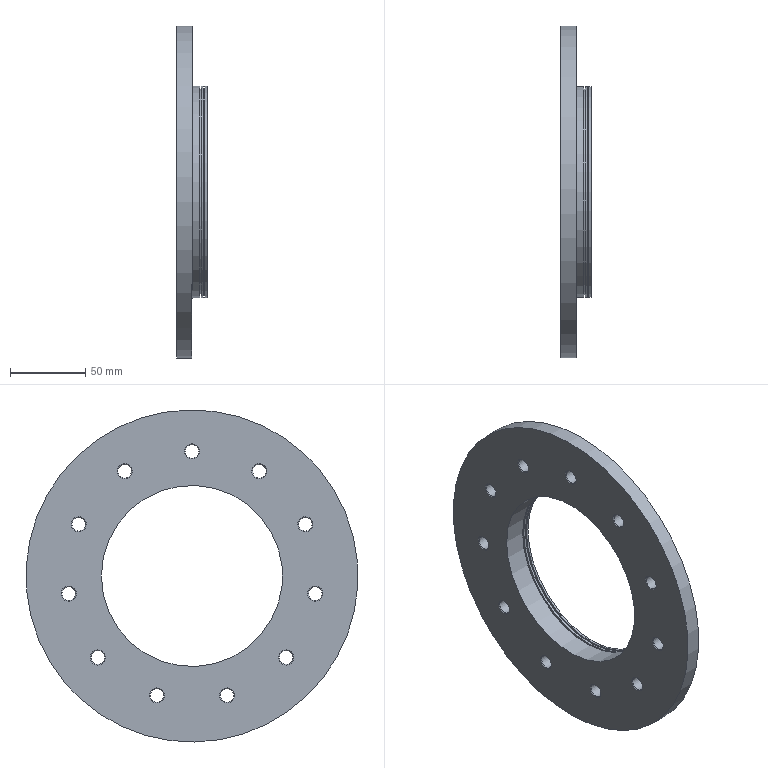Part | STEP file | Brake half | 1 solid | 46 faces | box 20 x 220 x 220 mm | volume 280546 mm3 | cylinder 23 | plane 12 | cone 11 | commonest cylinder face diameters 9 x11 120 x3 140 x3 124 x2 136 x2 177 x1
STEP:
#1=CARTESIAN_POINT('',(15.,0.,-70.));
#2=VERTEX_POINT('',#1);
#3=CARTESIAN_POINT('',(15.,0.,0.));
#4=DIRECTION('',(-1.,0.,0.));
#5=DIRECTION('',(0.,0.,-1.));
#6=AXIS2_PLACEMENT_3D('',#3,#4,#5);
#7=CIRCLE('',#6,70.);
#8=EDGE_CURVE('',#2,#2,#7,.T.);
#9=ORIENTED_EDGE('',*,*,#8,.T.);
#10=EDGE_LOOP('',(#9));
#11=FACE_OUTER_BOUND('',#10,.T.);
#12=CARTESIAN_POINT('',(8.,0.,-70.));
#13=VERTEX_POINT('',#12);
#14=CARTESIAN_POINT('',(8.,0.,0.));
#15=DIRECTION('',(1.,0.,0.));
#16=DIRECTION('',(0.,0.,-1.));
#17=AXIS2_PLACEMENT_3D('',#14,#15,#16);
#18=CIRCLE('',#17,70.);
#19=EDGE_CURVE('',#13,#13,#18,.T.);
#20=ORIENTED_EDGE('',*,*,#19,.T.);
#21=EDGE_LOOP('',(#20));
#22=FACE_OUTER_BOUND('',#21,.T.);
#23=CARTESIAN_POINT('',(20.,0.,0.));
#24=DIRECTION('',(-1.,0.,0.));
#25=DIRECTION('',(0.,0.,-1.));
#26=AXIS2_PLACEMENT_3D('',#23,#24,#25);
#27=CYLINDRICAL_SURFACE('',#26,70.);
#28=ADVANCED_FACE('',(#11,#22),#27,.T.);
#29=CARTESIAN_POINT('',(8.,-73.175,38.365));
#30=VERTEX_POINT('',#29);
#31=CARTESIAN_POINT('',(8.,-75.045,34.272));
#32=DIRECTION('',(1.,0.,0.));
#33=DIRECTION('',(0.,0.4154,0.9096));
#34=AXIS2_PLACEMENT_3D('',#31,#32,#33);
#35=CIRCLE('',#34,4.5);
#36=EDGE_CURVE('',#30,#30,#35,.T.);
#37=ORIENTED_EDGE('',*,*,#36,.T.);
#38=EDGE_LOOP('',(#37));
#39=FACE_OUTER_BOUND('',#38,.T.);
#40=CARTESIAN_POINT('',(0.5,-73.175,38.365));
#41=VERTEX_POINT('',#40);
#42=CARTESIAN_POINT('',(0.5,-75.045,34.272));
#43=DIRECTION('',(1.,0.,0.));
#44=DIRECTION('',(0.,0.4154,0.9096));
#45=AXIS2_PLACEMENT_3D('',#42,#43,#44);
#46=CIRCLE('',#45,4.5);
#47=EDGE_CURVE('',#41,#41,#46,.T.);
#48=ORIENTED_EDGE('',*,*,#47,.F.);
#49=EDGE_LOOP('',(#48));
#50=FACE_OUTER_BOUND('',#49,.T.);
#51=CARTESIAN_POINT('',(-30.,-75.045,34.272));
#52=DIRECTION('',(1.,0.,0.));
#53=DIRECTION('',(0.,0.4154,0.9096));
#54=AXIS2_PLACEMENT_3D('',#51,#52,#53);
#55=CYLINDRICAL_SURFACE('',#54,4.5);
#56=ADVANCED_FACE('',(#39,#50),#55,.F.);
#57=CARTESIAN_POINT('',(8.,-65.296,-50.625));
#58=VERTEX_POINT('',#57);
#59=CARTESIAN_POINT('',(8.,-62.349,-54.026));
#60=DIRECTION('',(1.,0.,0.));
#61=DIRECTION('',(0.,-0.6549,0.7557));
#62=AXIS2_PLACEMENT_3D('',#59,#60,#61);
#63=CIRCLE('',#62,4.5);
#64=EDGE_CURVE('',#58,#58,#63,.T.);
#65=ORIENTED_EDGE('',*,*,#64,.T.);
#66=EDGE_LOOP('',(#65));
#67=FACE_OUTER_BOUND('',#66,.T.);
#68=CARTESIAN_POINT('',(0.5,-65.296,-50.625));
#69=VERTEX_POINT('',#68);
#70=CARTESIAN_POINT('',(0.5,-62.349,-54.026));
#71=DIRECTION('',(1.,0.,0.));
#72=DIRECTION('',(0.,-0.6549,0.7557));
#73=AXIS2_PLACEMENT_3D('',#70,#71,#72);
#74=CIRCLE('',#73,4.5);
#75=EDGE_CURVE('',#69,#69,#74,.T.);
#76=ORIENTED_EDGE('',*,*,#75,.F.);
#77=EDGE_LOOP('',(#76));
#78=FACE_OUTER_BOUND('',#77,.T.);
#79=CARTESIAN_POINT('',(-30.,-62.349,-54.026));
#80=DIRECTION('',(1.,0.,0.));
#81=DIRECTION('',(0.,-0.6549,0.7557));
#82=AXIS2_PLACEMENT_3D('',#79,#80,#81);
#83=CYLINDRICAL_SURFACE('',#82,4.5);
#84=ADVANCED_FACE('',(#67,#78),#83,.F.);
#85=CARTESIAN_POINT('',(8.,18.925,-80.426));
#86=VERTEX_POINT('',#85);
#87=CARTESIAN_POINT('',(8.,23.243,-79.158));
#88=DIRECTION('',(1.,0.,0.));
#89=DIRECTION('',(0.,-0.9595,-0.2817));
#90=AXIS2_PLACEMENT_3D('',#87,#88,#89);
#91=CIRCLE('',#90,4.5);
#92=EDGE_CURVE('',#86,#86,#91,.T.);
#93=ORIENTED_EDGE('',*,*,#92,.T.);
#94=EDGE_LOOP('',(#93));
#95=FACE_OUTER_BOUND('',#94,.T.);
#96=CARTESIAN_POINT('',(0.5,18.925,-80.426));
#97=VERTEX_POINT('',#96);
#98=CARTESIAN_POINT('',(0.5,23.243,-79.158));
#99=DIRECTION('',(1.,0.,0.));
#100=DIRECTION('',(0.,-0.9595,-0.2817));
#101=AXIS2_PLACEMENT_3D('',#98,#99,#100);
#102=CIRCLE('',#101,4.5);
#103=EDGE_CURVE('',#97,#97,#102,.T.);
#104=ORIENTED_EDGE('',*,*,#103,.F.);
#105=EDGE_LOOP('',(#104));
#106=FACE_OUTER_BOUND('',#105,.T.);
#107=CARTESIAN_POINT('',(-30.,23.243,-79.158));
#108=DIRECTION('',(1.,0.,0.));
#109=DIRECTION('',(0.,-0.9595,-0.2817));
#110=AXIS2_PLACEMENT_3D('',#107,#108,#109);
#111=CYLINDRICAL_SURFACE('',#110,4.5);
#112=ADVANCED_FACE('',(#95,#106),#111,.F.);
#113=CARTESIAN_POINT('',(8.,81.02,-16.195));
#114=VERTEX_POINT('',#113);
#115=CARTESIAN_POINT('',(8.,81.66,-11.741));
#116=DIRECTION('',(1.,0.,0.));
#117=DIRECTION('',(0.,-0.1423,-0.9898));
#118=AXIS2_PLACEMENT_3D('',#115,#116,#117);
#119=CIRCLE('',#118,4.5);
#120=EDGE_CURVE('',#114,#114,#119,.T.);
#121=ORIENTED_EDGE('',*,*,#120,.T.);
#122=EDGE_LOOP('',(#121));
#123=FACE_OUTER_BOUND('',#122,.T.);
#124=CARTESIAN_POINT('',(0.5,81.02,-16.195));
#125=VERTEX_POINT('',#124);
#126=CARTESIAN_POINT('',(0.5,81.66,-11.741));
#127=DIRECTION('',(1.,0.,0.));
#128=DIRECTION('',(0.,-0.1423,-0.9898));
#129=AXIS2_PLACEMENT_3D('',#126,#127,#128);
#130=CIRCLE('',#129,4.5);
#131=EDGE_CURVE('',#125,#125,#130,.T.);
#132=ORIENTED_EDGE('',*,*,#131,.F.);
#133=EDGE_LOOP('',(#132));
#134=FACE_OUTER_BOUND('',#133,.T.);
#135=CARTESIAN_POINT('',(-30.,81.66,-11.741));
#136=DIRECTION('',(1.,0.,0.));
#137=DIRECTION('',(0.,-0.1423,-0.9898));
#138=AXIS2_PLACEMENT_3D('',#135,#136,#137);
#139=CYLINDRICAL_SURFACE('',#138,4.5);
#140=ADVANCED_FACE('',(#123,#134),#139,.F.);
#141=CARTESIAN_POINT('',(8.,48.389,66.971));
#142=VERTEX_POINT('',#141);
#143=CARTESIAN_POINT('',(8.,44.603,69.403));
#144=DIRECTION('',(1.,0.,0.));
#145=DIRECTION('',(0.,0.8413,-0.5406));
#146=AXIS2_PLACEMENT_3D('',#143,#144,#145);
#147=CIRCLE('',#146,4.5);
#148=EDGE_CURVE('',#142,#142,#147,.T.);
#149=ORIENTED_EDGE('',*,*,#148,.T.);
#150=EDGE_LOOP('',(#149));
#151=FACE_OUTER_BOUND('',#150,.T.);
#152=CARTESIAN_POINT('',(0.5,48.389,66.971));
#153=VERTEX_POINT('',#152);
#154=CARTESIAN_POINT('',(0.5,44.603,69.403));
#155=DIRECTION('',(1.,0.,0.));
#156=DIRECTION('',(0.,0.8413,-0.5406));
#157=AXIS2_PLACEMENT_3D('',#154,#155,#156);
#158=CIRCLE('',#157,4.5);
#159=EDGE_CURVE('',#153,#153,#158,.T.);
#160=ORIENTED_EDGE('',*,*,#159,.F.);
#161=EDGE_LOOP('',(#160));
#162=FACE_OUTER_BOUND('',#161,.T.);
#163=CARTESIAN_POINT('',(-30.,44.603,69.403));
#164=DIRECTION('',(1.,0.,0.));
#165=DIRECTION('',(0.,0.8413,-0.5406));
#166=AXIS2_PLACEMENT_3D('',#163,#164,#165);
#167=CYLINDRICAL_SURFACE('',#166,4.5);
#168=ADVANCED_FACE('',(#151,#162),#167,.F.);
#169=CARTESIAN_POINT('',(8.,76.914,30.178));
#170=VERTEX_POINT('',#169);
#171=CARTESIAN_POINT('',(8.,75.045,34.272));
#172=DIRECTION('',(1.,0.,0.));
#173=DIRECTION('',(0.,0.4154,-0.9096));
#174=AXIS2_PLACEMENT_3D('',#171,#172,#173);
#175=CIRCLE('',#174,4.5);
#176=EDGE_CURVE('',#170,#170,#175,.T.);
#177=ORIENTED_EDGE('',*,*,#176,.T.);
#178=EDGE_LOOP('',(#177));
#179=FACE_OUTER_BOUND('',#178,.T.);
#180=CARTESIAN_POINT('',(0.5,76.914,30.178));
#181=VERTEX_POINT('',#180);
#182=CARTESIAN_POINT('',(0.5,75.045,34.272));
#183=DIRECTION('',(1.,0.,0.));
#184=DIRECTION('',(0.,0.4154,-0.9096));
#185=AXIS2_PLACEMENT_3D('',#182,#183,#184);
#186=CIRCLE('',#185,4.5);
#187=EDGE_CURVE('',#181,#181,#186,.T.);
#188=ORIENTED_EDGE('',*,*,#187,.F.);
#189=EDGE_LOOP('',(#188));
#190=FACE_OUTER_BOUND('',#189,.T.);
#191=CARTESIAN_POINT('',(-30.,75.045,34.272));
#192=DIRECTION('',(1.,0.,0.));
#193=DIRECTION('',(0.,0.4154,-0.9096));
#194=AXIS2_PLACEMENT_3D('',#191,#192,#193);
#195=CYLINDRICAL_SURFACE('',#194,4.5);
#196=ADVANCED_FACE('',(#179,#190),#195,.F.);
#197=CARTESIAN_POINT('',(8.,59.402,-57.427));
#198=VERTEX_POINT('',#197);
#199=CARTESIAN_POINT('',(8.,62.349,-54.026));
#200=DIRECTION('',(1.,0.,0.));
#201=DIRECTION('',(0.,-0.6549,-0.7557));
#202=AXIS2_PLACEMENT_3D('',#199,#200,#201);
#203=CIRCLE('',#202,4.5);
#204=EDGE_CURVE('',#198,#198,#203,.T.);
#205=ORIENTED_EDGE('',*,*,#204,.T.);
#206=EDGE_LOOP('',(#205));
#207=FACE_OUTER_BOUND('',#206,.T.);
#208=CARTESIAN_POINT('',(0.5,59.402,-57.427));
#209=VERTEX_POINT('',#208);
#210=CARTESIAN_POINT('',(0.5,62.349,-54.026));
#211=DIRECTION('',(1.,0.,0.));
#212=DIRECTION('',(0.,-0.6549,-0.7557));
#213=AXIS2_PLACEMENT_3D('',#210,#211,#212);
#214=CIRCLE('',#213,4.5);
#215=EDGE_CURVE('',#209,#209,#214,.T.);
#216=ORIENTED_EDGE('',*,*,#215,.F.);
#217=EDGE_LOOP('',(#216));
#218=FACE_OUTER_BOUND('',#217,.T.);
#219=CARTESIAN_POINT('',(-30.,62.349,-54.026));
#220=DIRECTION('',(1.,0.,0.));
#221=DIRECTION('',(0.,-0.6549,-0.7557));
#222=AXIS2_PLACEMENT_3D('',#219,#220,#221);
#223=CYLINDRICAL_SURFACE('',#222,4.5);
#224=ADVANCED_FACE('',(#207,#218),#223,.F.);
#225=CARTESIAN_POINT('',(8.,-27.561,-77.89));
#226=VERTEX_POINT('',#225);
#227=CARTESIAN_POINT('',(8.,-23.243,-79.158));
#228=DIRECTION('',(1.,0.,0.));
#229=DIRECTION('',(0.,-0.9595,0.2817));
#230=AXIS2_PLACEMENT_3D('',#227,#228,#229);
#231=CIRCLE('',#230,4.5);
#232=EDGE_CURVE('',#226,#226,#231,.T.);
#233=ORIENTED_EDGE('',*,*,#232,.T.);
#234=EDGE_LOOP('',(#233));
#235=FACE_OUTER_BOUND('',#234,.T.);
#236=CARTESIAN_POINT('',(0.5,-27.561,-77.89));
#237=VERTEX_POINT('',#236);
#238=CARTESIAN_POINT('',(0.5,-23.243,-79.158));
#239=DIRECTION('',(1.,0.,0.));
#240=DIRECTION('',(0.,-0.9595,0.2817));
#241=AXIS2_PLACEMENT_3D('',#238,#239,#240);
#242=CIRCLE('',#241,4.5);
#243=EDGE_CURVE('',#237,#237,#242,.T.);
#244=ORIENTED_EDGE('',*,*,#243,.F.);
#245=EDGE_LOOP('',(#244));
#246=FACE_OUTER_BOUND('',#245,.T.);
#247=CARTESIAN_POINT('',(-30.,-23.243,-79.158));
#248=DIRECTION('',(1.,0.,0.));
#249=DIRECTION('',(0.,-0.9595,0.2817));
#250=AXIS2_PLACEMENT_3D('',#247,#248,#249);
#251=CYLINDRICAL_SURFACE('',#250,4.5);
#252=ADVANCED_FACE('',(#235,#246),#251,.F.);
#253=CARTESIAN_POINT('',(8.,-82.301,-7.287));
#254=VERTEX_POINT('',#253);
#255=CARTESIAN_POINT('',(8.,-81.66,-11.741));
#256=DIRECTION('',(1.,0.,0.));
#257=DIRECTION('',(0.,-0.1423,0.9898));
#258=AXIS2_PLACEMENT_3D('',#255,#256,#257);
#259=CIRCLE('',#258,4.5);
#260=EDGE_CURVE('',#254,#254,#259,.T.);
#261=ORIENTED_EDGE('',*,*,#260,.T.);
#262=EDGE_LOOP('',(#261));
#263=FACE_OUTER_BOUND('',#262,.T.);
#264=CARTESIAN_POINT('',(0.5,-82.301,-7.287));
#265=VERTEX_POINT('',#264);
#266=CARTESIAN_POINT('',(0.5,-81.66,-11.741));
#267=DIRECTION('',(1.,0.,0.));
#268=DIRECTION('',(0.,-0.1423,0.9898));
#269=AXIS2_PLACEMENT_3D('',#266,#267,#268);
#270=CIRCLE('',#269,4.5);
#271=EDGE_CURVE('',#265,#265,#270,.T.);
#272=ORIENTED_EDGE('',*,*,#271,.F.);
#273=EDGE_LOOP('',(#272));
#274=FACE_OUTER_BOUND('',#273,.T.);
#275=CARTESIAN_POINT('',(-30.,-81.66,-11.741));
#276=DIRECTION('',(1.,0.,0.));
#277=DIRECTION('',(0.,-0.1423,0.9898));
#278=AXIS2_PLACEMENT_3D('',#275,#276,#277);
#279=CYLINDRICAL_SURFACE('',#278,4.5);
#280=ADVANCED_FACE('',(#263,#274),#279,.F.);
#281=CARTESIAN_POINT('',(8.,-40.817,71.836));
#282=VERTEX_POINT('',#281);
#283=CARTESIAN_POINT('',(8.,-44.603,69.403));
#284=DIRECTION('',(1.,0.,0.));
#285=DIRECTION('',(0.,0.8413,0.5406));
#286=AXIS2_PLACEMENT_3D('',#283,#284,#285);
#287=CIRCLE('',#286,4.5);
#288=EDGE_CURVE('',#282,#282,#287,.T.);
#289=ORIENTED_EDGE('',*,*,#288,.T.);
#290=EDGE_LOOP('',(#289));
#291=FACE_OUTER_BOUND('',#290,.T.);
#292=CARTESIAN_POINT('',(0.5,-40.817,71.836));
#293=VERTEX_POINT('',#292);
#294=CARTESIAN_POINT('',(0.5,-44.603,69.403));
#295=DIRECTION('',(1.,0.,0.));
#296=DIRECTION('',(0.,0.8413,0.5406));
#297=AXIS2_PLACEMENT_3D('',#294,#295,#296);
#298=CIRCLE('',#297,4.5);
#299=EDGE_CURVE('',#293,#293,#298,.T.);
#300=ORIENTED_EDGE('',*,*,#299,.F.);
#301=EDGE_LOOP('',(#300));
#302=FACE_OUTER_BOUND('',#301,.T.);
#303=CARTESIAN_POINT('',(-30.,-44.603,69.403));
#304=DIRECTION('',(1.,0.,0.));
#305=DIRECTION('',(0.,0.8413,0.5406));
#306=AXIS2_PLACEMENT_3D('',#303,#304,#305);
#307=CYLINDRICAL_SURFACE('',#306,4.5);
#308=ADVANCED_FACE('',(#291,#302),#307,.F.);
#309=CARTESIAN_POINT('',(8.,4.5,82.5));
#310=VERTEX_POINT('',#309);
#311=CARTESIAN_POINT('',(8.,0.,82.5));
#312=DIRECTION('',(1.,0.,0.));
#313=DIRECTION('',(0.,1.,0.));
#314=AXIS2_PLACEMENT_3D('',#311,#312,#313);
#315=CIRCLE('',#314,4.5);
#316=EDGE_CURVE('',#310,#310,#315,.T.);
#317=ORIENTED_EDGE('',*,*,#316,.T.);
#318=EDGE_LOOP('',(#317));
#319=FACE_OUTER_BOUND('',#318,.T.);
#320=CARTESIAN_POINT('',(0.5,4.5,82.5));
#321=VERTEX_POINT('',#320);
#322=CARTESIAN_POINT('',(0.5,0.,82.5));
#323=DIRECTION('',(1.,0.,0.));
#324=DIRECTION('',(0.,1.,0.));
#325=AXIS2_PLACEMENT_3D('',#322,#323,#324);
#326=CIRCLE('',#325,4.5);
#327=EDGE_CURVE('',#321,#321,#326,.T.);
#328=ORIENTED_EDGE('',*,*,#327,.F.);
#329=EDGE_LOOP('',(#328));
#330=FACE_OUTER_BOUND('',#329,.T.);
#331=CARTESIAN_POINT('',(-30.,0.,82.5));
#332=DIRECTION('',(1.,0.,0.));
#333=DIRECTION('',(0.,1.,0.));
#334=AXIS2_PLACEMENT_3D('',#331,#332,#333);
#335=CYLINDRICAL_SURFACE('',#334,4.5);
#336=ADVANCED_FACE('',(#319,#330),#335,.F.);
#337=CARTESIAN_POINT('',(10.,-109.545,10.));
#338=VERTEX_POINT('',#337);
#339=CARTESIAN_POINT('',(10.,0.,0.));
#340=DIRECTION('',(1.,0.,0.));
#341=DIRECTION('',(0.,0.,-1.));
#342=AXIS2_PLACEMENT_3D('',#339,#340,#341);
#343=CIRCLE('',#342,110.);
#344=EDGE_CURVE('',#338,#338,#343,.T.);
#345=ORIENTED_EDGE('',*,*,#344,.T.);
#346=EDGE_LOOP('',(#345));
#347=FACE_BOUND('',#346,.T.);
#348=CARTESIAN_POINT('',(10.,0.,-88.5));
#349=VERTEX_POINT('',#348);
#350=CARTESIAN_POINT('',(10.,0.,0.));
#351=DIRECTION('',(1.,0.,0.));
#352=DIRECTION('',(0.,0.,-1.));
#353=AXIS2_PLACEMENT_3D('',#350,#351,#352);
#354=CIRCLE('',#353,88.5);
#355=EDGE_CURVE('',#349,#349,#354,.F.);
#356=ORIENTED_EDGE('',*,*,#355,.T.);
#357=EDGE_LOOP('',(#356));
#358=FACE_BOUND('',#357,.T.);
#359=CARTESIAN_POINT('',(10.,0.,0.));
#360=DIRECTION('',(1.,0.,0.));
#361=DIRECTION('',(0.,0.,-1.));
#362=AXIS2_PLACEMENT_3D('',#359,#360,#361);
#363=PLANE('',#362);
#364=ADVANCED_FACE('',(#347,#358),#363,.T.);
#365=ORIENTED_EDGE('',*,*,#355,.F.);
#366=EDGE_LOOP('',(#365));
#367=FACE_OUTER_BOUND('',#366,.T.);
#368=CARTESIAN_POINT('',(8.,0.,-88.5));
#369=VERTEX_POINT('',#368);
#370=CARTESIAN_POINT('',(8.,0.,0.));
#371=DIRECTION('',(1.,0.,0.));
#372=DIRECTION('',(0.,0.,-1.));
#373=AXIS2_PLACEMENT_3D('',#370,#371,#372);
#374=CIRCLE('',#373,88.5);
#375=EDGE_CURVE('',#369,#369,#374,.T.);
#376=ORIENTED_EDGE('',*,*,#375,.F.);
#377=EDGE_LOOP('',(#376));
#378=FACE_OUTER_BOUND('',#377,.T.);
#379=CARTESIAN_POINT('',(8.,0.,0.));
#380=DIRECTION('',(1.,0.,0.));
#381=DIRECTION('',(0.,0.,-1.));
#382=AXIS2_PLACEMENT_3D('',#379,#380,#381);
#383=CYLINDRICAL_SURFACE('',#382,88.5);
#384=ADVANCED_FACE('',(#367,#378),#383,.F.);
#385=ORIENTED_EDGE('',*,*,#375,.T.);
#386=EDGE_LOOP('',(#385));
#387=FACE_BOUND('',#386,.T.);
#388=ORIENTED_EDGE('',*,*,#316,.F.);
#389=EDGE_LOOP('',(#388));
#390=FACE_BOUND('',#389,.T.);
#391=ORIENTED_EDGE('',*,*,#288,.F.);
#392=EDGE_LOOP('',(#391));
#393=FACE_BOUND('',#392,.T.);
#394=ORIENTED_EDGE('',*,*,#260,.F.);
#395=EDGE_LOOP('',(#394));
#396=FACE_BOUND('',#395,.T.);
#397=ORIENTED_EDGE('',*,*,#232,.F.);
#398=EDGE_LOOP('',(#397));
#399=FACE_BOUND('',#398,.T.);
#400=ORIENTED_EDGE('',*,*,#204,.F.);
#401=EDGE_LOOP('',(#400));
#402=FACE_BOUND('',#401,.T.);
#403=ORIENTED_EDGE('',*,*,#176,.F.);
#404=EDGE_LOOP('',(#403));
#405=FACE_BOUND('',#404,.T.);
#406=ORIENTED_EDGE('',*,*,#148,.F.);
#407=EDGE_LOOP('',(#406));
#408=FACE_BOUND('',#407,.T.);
#409=ORIENTED_EDGE('',*,*,#120,.F.);
#410=EDGE_LOOP('',(#409));
#411=FACE_BOUND('',#410,.T.);
#412=ORIENTED_EDGE('',*,*,#92,.F.);
#413=EDGE_LOOP('',(#412));
#414=FACE_BOUND('',#413,.T.);
#415=ORIENTED_EDGE('',*,*,#64,.F.);
#416=EDGE_LOOP('',(#415));
#417=FACE_BOUND('',#416,.T.);
#418=ORIENTED_EDGE('',*,*,#36,.F.);
#419=EDGE_LOOP('',(#418));
#420=FACE_BOUND('',#419,.T.);
#421=ORIENTED_EDGE('',*,*,#19,.F.);
#422=EDGE_LOOP('',(#421));
#423=FACE_BOUND('',#422,.T.);
#424=CARTESIAN_POINT('',(8.,0.,0.));
#425=DIRECTION('',(1.,0.,0.));
#426=DIRECTION('',(0.,0.,-1.));
#427=AXIS2_PLACEMENT_3D('',#424,#425,#426);
#428=PLANE('',#427);
#429=ADVANCED_FACE('',(#387,#390,#393,#396,#399,#402,#405,#408,#411,#414,#417,#420,#423),#428,.T.);
#430=ORIENTED_EDGE('',*,*,#8,.F.);
#431=EDGE_LOOP('',(#430));
#432=FACE_BOUND('',#431,.T.);
#433=CARTESIAN_POINT('',(15.,0.,68.));
#434=VERTEX_POINT('',#433);
#435=CARTESIAN_POINT('',(15.,0.,0.));
#436=DIRECTION('',(-1.,0.,0.));
#437=DIRECTION('',(0.,0.,1.));
#438=AXIS2_PLACEMENT_3D('',#435,#436,#437);
#439=CIRCLE('',#438,68.);
#440=EDGE_CURVE('',#434,#434,#439,.T.);
#441=ORIENTED_EDGE('',*,*,#440,.T.);
#442=EDGE_LOOP('',(#441));
#443=FACE_BOUND('',#442,.T.);
#444=CARTESIAN_POINT('',(15.,0.,0.));
#445=DIRECTION('',(-1.,0.,0.));
#446=DIRECTION('',(0.,0.,1.));
#447=AXIS2_PLACEMENT_3D('',#444,#445,#446);
#448=PLANE('',#447);
#449=ADVANCED_FACE('',(#432,#443),#448,.F.);
#450=ORIENTED_EDGE('',*,*,#47,.T.);
#451=EDGE_LOOP('',(#450));
#452=FACE_OUTER_BOUND('',#451,.T.);
#453=CARTESIAN_POINT('',(0.,-72.968,38.82));
#454=VERTEX_POINT('',#453);
#455=CARTESIAN_POINT('',(0.,-75.045,34.272));
#456=DIRECTION('',(1.,0.,0.));
#457=DIRECTION('',(0.,0.4154,0.9096));
#458=AXIS2_PLACEMENT_3D('',#455,#456,#457);
#459=CIRCLE('',#458,5.);
#460=EDGE_CURVE('',#454,#454,#459,.T.);
#461=ORIENTED_EDGE('',*,*,#460,.F.);
#462=EDGE_LOOP('',(#461));
#463=FACE_OUTER_BOUND('',#462,.T.);
#464=CARTESIAN_POINT('',(0.25,-75.045,34.272));
#465=DIRECTION('',(-1.,0.,0.));
#466=DIRECTION('',(0.,-0.4154,-0.9096));
#467=AXIS2_PLACEMENT_3D('',#464,#465,#466);
#468=CONICAL_SURFACE('',#467,4.75,0.7854);
#469=ADVANCED_FACE('',(#452,#463),#468,.F.);
#470=ORIENTED_EDGE('',*,*,#75,.T.);
#471=EDGE_LOOP('',(#470));
#472=FACE_OUTER_BOUND('',#471,.T.);
#473=CARTESIAN_POINT('',(0.,-65.624,-50.247));
#474=VERTEX_POINT('',#473);
#475=CARTESIAN_POINT('',(0.,-62.349,-54.026));
#476=DIRECTION('',(1.,0.,0.));
#477=DIRECTION('',(0.,-0.6549,0.7557));
#478=AXIS2_PLACEMENT_3D('',#475,#476,#477);
#479=CIRCLE('',#478,5.);
#480=EDGE_CURVE('',#474,#474,#479,.T.);
#481=ORIENTED_EDGE('',*,*,#480,.F.);
#482=EDGE_LOOP('',(#481));
#483=FACE_OUTER_BOUND('',#482,.T.);
#484=CARTESIAN_POINT('',(0.25,-62.349,-54.026));
#485=DIRECTION('',(-1.,0.,0.));
#486=DIRECTION('',(0.,0.6549,-0.7557));
#487=AXIS2_PLACEMENT_3D('',#484,#485,#486);
#488=CONICAL_SURFACE('',#487,4.75,0.7854);
#489=ADVANCED_FACE('',(#472,#483),#488,.F.);
#490=ORIENTED_EDGE('',*,*,#103,.T.);
#491=EDGE_LOOP('',(#490));
#492=FACE_OUTER_BOUND('',#491,.T.);
#493=CARTESIAN_POINT('',(0.,18.445,-80.567));
#494=VERTEX_POINT('',#493);
#495=CARTESIAN_POINT('',(0.,23.243,-79.158));
#496=DIRECTION('',(1.,0.,0.));
#497=DIRECTION('',(0.,-0.9595,-0.2817));
#498=AXIS2_PLACEMENT_3D('',#495,#496,#497);
#499=CIRCLE('',#498,5.);
#500=EDGE_CURVE('',#494,#494,#499,.T.);
#501=ORIENTED_EDGE('',*,*,#500,.F.);
#502=EDGE_LOOP('',(#501));
#503=FACE_OUTER_BOUND('',#502,.T.);
#504=CARTESIAN_POINT('',(0.25,23.243,-79.158));
#505=DIRECTION('',(-1.,0.,0.));
#506=DIRECTION('',(0.,0.9595,0.2817));
#507=AXIS2_PLACEMENT_3D('',#504,#505,#506);
#508=CONICAL_SURFACE('',#507,4.75,0.7854);
#509=ADVANCED_FACE('',(#492,#503),#508,.F.);
#510=ORIENTED_EDGE('',*,*,#131,.T.);
#511=EDGE_LOOP('',(#510));
#512=FACE_OUTER_BOUND('',#511,.T.);
#513=CARTESIAN_POINT('',(0.,80.949,-16.69));
#514=VERTEX_POINT('',#513);
#515=CARTESIAN_POINT('',(0.,81.66,-11.741));
#516=DIRECTION('',(1.,0.,0.));
#517=DIRECTION('',(0.,-0.1423,-0.9898));
#518=AXIS2_PLACEMENT_3D('',#515,#516,#517);
#519=CIRCLE('',#518,5.);
#520=EDGE_CURVE('',#514,#514,#519,.T.);
#521=ORIENTED_EDGE('',*,*,#520,.F.);
#522=EDGE_LOOP('',(#521));
#523=FACE_OUTER_BOUND('',#522,.T.);
#524=CARTESIAN_POINT('',(0.25,81.66,-11.741));
#525=DIRECTION('',(-1.,0.,0.));
#526=DIRECTION('',(0.,0.1423,0.9898));
#527=AXIS2_PLACEMENT_3D('',#524,#525,#526);
#528=CONICAL_SURFACE('',#527,4.75,0.7854);
#529=ADVANCED_FACE('',(#512,#523),#528,.F.);
#530=ORIENTED_EDGE('',*,*,#159,.T.);
#531=EDGE_LOOP('',(#530));
#532=FACE_OUTER_BOUND('',#531,.T.);
#533=CARTESIAN_POINT('',(0.,48.809,66.7));
#534=VERTEX_POINT('',#533);
#535=CARTESIAN_POINT('',(0.,44.603,69.403));
#536=DIRECTION('',(1.,0.,0.));
#537=DIRECTION('',(0.,0.8413,-0.5406));
#538=AXIS2_PLACEMENT_3D('',#535,#536,#537);
#539=CIRCLE('',#538,5.);
#540=EDGE_CURVE('',#534,#534,#539,.T.);
#541=ORIENTED_EDGE('',*,*,#540,.F.);
#542=EDGE_LOOP('',(#541));
#543=FACE_OUTER_BOUND('',#542,.T.);
#544=CARTESIAN_POINT('',(0.25,44.603,69.403));
#545=DIRECTION('',(-1.,0.,0.));
#546=DIRECTION('',(0.,-0.8413,0.5406));
#547=AXIS2_PLACEMENT_3D('',#544,#545,#546);
#548=CONICAL_SURFACE('',#547,4.75,0.7854);
#549=ADVANCED_FACE('',(#532,#543),#548,.F.);
#550=ORIENTED_EDGE('',*,*,#187,.T.);
#551=EDGE_LOOP('',(#550));
#552=FACE_OUTER_BOUND('',#551,.T.);
#553=CARTESIAN_POINT('',(0.,77.122,29.724));
#554=VERTEX_POINT('',#553);
#555=CARTESIAN_POINT('',(0.,75.045,34.272));
#556=DIRECTION('',(1.,0.,0.));
#557=DIRECTION('',(0.,0.4154,-0.9096));
#558=AXIS2_PLACEMENT_3D('',#555,#556,#557);
#559=CIRCLE('',#558,5.);
#560=EDGE_CURVE('',#554,#554,#559,.T.);
#561=ORIENTED_EDGE('',*,*,#560,.F.);
#562=EDGE_LOOP('',(#561));
#563=FACE_OUTER_BOUND('',#562,.T.);
#564=CARTESIAN_POINT('',(0.25,75.045,34.272));
#565=DIRECTION('',(-1.,0.,0.));
#566=DIRECTION('',(0.,-0.4154,0.9096));
#567=AXIS2_PLACEMENT_3D('',#564,#565,#566);
#568=CONICAL_SURFACE('',#567,4.75,0.7854);
#569=ADVANCED_FACE('',(#552,#563),#568,.F.);
#570=ORIENTED_EDGE('',*,*,#215,.T.);
#571=EDGE_LOOP('',(#570));
#572=FACE_OUTER_BOUND('',#571,.T.);
#573=CARTESIAN_POINT('',(0.,59.075,-57.805));
#574=VERTEX_POINT('',#573);
#575=CARTESIAN_POINT('',(0.,62.349,-54.026));
#576=DIRECTION('',(1.,0.,0.));
#577=DIRECTION('',(0.,-0.6549,-0.7557));
#578=AXIS2_PLACEMENT_3D('',#575,#576,#577);
#579=CIRCLE('',#578,5.);
#580=EDGE_CURVE('',#574,#574,#579,.T.);
#581=ORIENTED_EDGE('',*,*,#580,.F.);
#582=EDGE_LOOP('',(#581));
#583=FACE_OUTER_BOUND('',#582,.T.);
#584=CARTESIAN_POINT('',(0.25,62.349,-54.026));
#585=DIRECTION('',(-1.,0.,0.));
#586=DIRECTION('',(0.,0.6549,0.7557));
#587=AXIS2_PLACEMENT_3D('',#584,#585,#586);
#588=CONICAL_SURFACE('',#587,4.75,0.7854);
#589=ADVANCED_FACE('',(#572,#583),#588,.F.);
#590=ORIENTED_EDGE('',*,*,#243,.T.);
#591=EDGE_LOOP('',(#590));
#592=FACE_OUTER_BOUND('',#591,.T.);
#593=CARTESIAN_POINT('',(0.,-28.04,-77.75));
#594=VERTEX_POINT('',#593);
#595=CARTESIAN_POINT('',(0.,-23.243,-79.158));
#596=DIRECTION('',(1.,0.,0.));
#597=DIRECTION('',(0.,-0.9595,0.2817));
#598=AXIS2_PLACEMENT_3D('',#595,#596,#597);
#599=CIRCLE('',#598,5.);
#600=EDGE_CURVE('',#594,#594,#599,.T.);
#601=ORIENTED_EDGE('',*,*,#600,.F.);
#602=EDGE_LOOP('',(#601));
#603=FACE_OUTER_BOUND('',#602,.T.);
#604=CARTESIAN_POINT('',(0.25,-23.243,-79.158));
#605=DIRECTION('',(-1.,0.,0.));
#606=DIRECTION('',(0.,0.9595,-0.2817));
#607=AXIS2_PLACEMENT_3D('',#604,#605,#606);
#608=CONICAL_SURFACE('',#607,4.75,0.7854);
#609=ADVANCED_FACE('',(#592,#603),#608,.F.);
#610=ORIENTED_EDGE('',*,*,#271,.T.);
#611=EDGE_LOOP('',(#610));
#612=FACE_OUTER_BOUND('',#611,.T.);
#613=CARTESIAN_POINT('',(0.,-82.372,-6.792));
#614=VERTEX_POINT('',#613);
#615=CARTESIAN_POINT('',(0.,-81.66,-11.741));
#616=DIRECTION('',(1.,0.,0.));
#617=DIRECTION('',(0.,-0.1423,0.9898));
#618=AXIS2_PLACEMENT_3D('',#615,#616,#617);
#619=CIRCLE('',#618,5.);
#620=EDGE_CURVE('',#614,#614,#619,.T.);
#621=ORIENTED_EDGE('',*,*,#620,.F.);
#622=EDGE_LOOP('',(#621));
#623=FACE_OUTER_BOUND('',#622,.T.);
#624=CARTESIAN_POINT('',(0.25,-81.66,-11.741));
#625=DIRECTION('',(-1.,0.,0.));
#626=DIRECTION('',(0.,0.1423,-0.9898));
#627=AXIS2_PLACEMENT_3D('',#624,#625,#626);
#628=CONICAL_SURFACE('',#627,4.75,0.7854);
#629=ADVANCED_FACE('',(#612,#623),#628,.F.);
#630=ORIENTED_EDGE('',*,*,#299,.T.);
#631=EDGE_LOOP('',(#630));
#632=FACE_OUTER_BOUND('',#631,.T.);
#633=CARTESIAN_POINT('',(0.,-40.397,72.107));
#634=VERTEX_POINT('',#633);
#635=CARTESIAN_POINT('',(0.,-44.603,69.403));
#636=DIRECTION('',(1.,0.,0.));
#637=DIRECTION('',(0.,0.8413,0.5406));
#638=AXIS2_PLACEMENT_3D('',#635,#636,#637);
#639=CIRCLE('',#638,5.);
#640=EDGE_CURVE('',#634,#634,#639,.T.);
#641=ORIENTED_EDGE('',*,*,#640,.F.);
#642=EDGE_LOOP('',(#641));
#643=FACE_OUTER_BOUND('',#642,.T.);
#644=CARTESIAN_POINT('',(0.25,-44.603,69.403));
#645=DIRECTION('',(-1.,0.,0.));
#646=DIRECTION('',(0.,-0.8413,-0.5406));
#647=AXIS2_PLACEMENT_3D('',#644,#645,#646);
#648=CONICAL_SURFACE('',#647,4.75,0.7854);
#649=ADVANCED_FACE('',(#632,#643),#648,.F.);
#650=ORIENTED_EDGE('',*,*,#327,.T.);
#651=EDGE_LOOP('',(#650));
#652=FACE_OUTER_BOUND('',#651,.T.);
#653=CARTESIAN_POINT('',(0.,5.,82.5));
#654=VERTEX_POINT('',#653);
#655=CARTESIAN_POINT('',(0.,0.,82.5));
#656=DIRECTION('',(1.,0.,0.));
#657=DIRECTION('',(0.,1.,0.));
#658=AXIS2_PLACEMENT_3D('',#655,#656,#657);
#659=CIRCLE('',#658,5.);
#660=EDGE_CURVE('',#654,#654,#659,.T.);
#661=ORIENTED_EDGE('',*,*,#660,.F.);
#662=EDGE_LOOP('',(#661));
#663=FACE_OUTER_BOUND('',#662,.T.);
#664=CARTESIAN_POINT('',(0.25,0.,82.5));
#665=DIRECTION('',(-1.,0.,0.));
#666=DIRECTION('',(0.,-1.,0.));
#667=AXIS2_PLACEMENT_3D('',#664,#665,#666);
#668=CONICAL_SURFACE('',#667,4.75,0.7854);
#669=ADVANCED_FACE('',(#652,#663),#668,.F.);
#670=ORIENTED_EDGE('',*,*,#344,.F.);
#671=EDGE_LOOP('',(#670));
#672=FACE_OUTER_BOUND('',#671,.T.);
#673=CARTESIAN_POINT('',(0.,-109.545,10.));
#674=VERTEX_POINT('',#673);
#675=CARTESIAN_POINT('',(0.,0.,0.));
#676=DIRECTION('',(1.,0.,0.));
#677=DIRECTION('',(0.,0.,-1.));
#678=AXIS2_PLACEMENT_3D('',#675,#676,#677);
#679=CIRCLE('',#678,110.);
#680=EDGE_CURVE('',#674,#674,#679,.T.);
#681=ORIENTED_EDGE('',*,*,#680,.T.);
#682=EDGE_LOOP('',(#681));
#683=FACE_OUTER_BOUND('',#682,.T.);
#684=CARTESIAN_POINT('',(0.,0.,0.));
#685=DIRECTION('',(1.,0.,0.));
#686=DIRECTION('',(0.,-0.9959,0.09091));
#687=AXIS2_PLACEMENT_3D('',#684,#685,#686);
#688=CYLINDRICAL_SURFACE('',#687,110.);
#689=ADVANCED_FACE('',(#672,#683),#688,.T.);
#690=CARTESIAN_POINT('',(16.,0.,68.));
#691=VERTEX_POINT('',#690);
#692=CARTESIAN_POINT('',(16.,0.,0.));
#693=DIRECTION('',(-1.,0.,0.));
#694=DIRECTION('',(0.,0.,1.));
#695=AXIS2_PLACEMENT_3D('',#692,#693,#694);
#696=CIRCLE('',#695,68.);
#697=EDGE_CURVE('',#691,#691,#696,.T.);
#698=ORIENTED_EDGE('',*,*,#697,.T.);
#699=EDGE_LOOP('',(#698));
#700=FACE_OUTER_BOUND('',#699,.T.);
#701=ORIENTED_EDGE('',*,*,#440,.F.);
#702=EDGE_LOOP('',(#701));
#703=FACE_OUTER_BOUND('',#702,.T.);
#704=CARTESIAN_POINT('',(15.,0.,0.));
#705=DIRECTION('',(-1.,0.,0.));
#706=DIRECTION('',(0.,0.,1.));
#707=AXIS2_PLACEMENT_3D('',#704,#705,#706);
#708=CYLINDRICAL_SURFACE('',#707,68.);
#709=ADVANCED_FACE('',(#700,#703),#708,.T.);
#710=ORIENTED_EDGE('',*,*,#680,.F.);
#711=EDGE_LOOP('',(#710));
#712=FACE_BOUND('',#711,.T.);
#713=ORIENTED_EDGE('',*,*,#660,.T.);
#714=EDGE_LOOP('',(#713));
#715=FACE_BOUND('',#714,.T.);
#716=ORIENTED_EDGE('',*,*,#560,.T.);
#717=EDGE_LOOP('',(#716));
#718=FACE_BOUND('',#717,.T.);
#719=ORIENTED_EDGE('',*,*,#580,.T.);
#720=EDGE_LOOP('',(#719));
#721=FACE_BOUND('',#720,.T.);
#722=ORIENTED_EDGE('',*,*,#600,.T.);
#723=EDGE_LOOP('',(#722));
#724=FACE_BOUND('',#723,.T.);
#725=ORIENTED_EDGE('',*,*,#620,.T.);
#726=EDGE_LOOP('',(#725));
#727=FACE_BOUND('',#726,.T.);
#728=ORIENTED_EDGE('',*,*,#640,.T.);
#729=EDGE_LOOP('',(#728));
#730=FACE_BOUND('',#729,.T.);
#731=CARTESIAN_POINT('',(0.,60.,0.));
#732=VERTEX_POINT('',#731);
#733=CARTESIAN_POINT('',(0.,0.,0.));
#734=DIRECTION('',(1.,0.,0.));
#735=DIRECTION('',(0.,1.,0.));
#736=AXIS2_PLACEMENT_3D('',#733,#734,#735);
#737=CIRCLE('',#736,60.);
#738=EDGE_CURVE('',#732,#732,#737,.T.);
#739=ORIENTED_EDGE('',*,*,#738,.T.);
#740=EDGE_LOOP('',(#739));
#741=FACE_BOUND('',#740,.T.);
#742=ORIENTED_EDGE('',*,*,#460,.T.);
#743=EDGE_LOOP('',(#742));
#744=FACE_BOUND('',#743,.T.);
#745=ORIENTED_EDGE('',*,*,#480,.T.);
#746=EDGE_LOOP('',(#745));
#747=FACE_BOUND('',#746,.T.);
#748=ORIENTED_EDGE('',*,*,#500,.T.);
#749=EDGE_LOOP('',(#748));
#750=FACE_BOUND('',#749,.T.);
#751=ORIENTED_EDGE('',*,*,#520,.T.);
#752=EDGE_LOOP('',(#751));
#753=FACE_BOUND('',#752,.T.);
#754=ORIENTED_EDGE('',*,*,#540,.T.);
#755=EDGE_LOOP('',(#754));
#756=FACE_BOUND('',#755,.T.);
#757=CARTESIAN_POINT('',(0.,0.,0.));
#758=DIRECTION('',(1.,0.,0.));
#759=DIRECTION('',(0.,0.,-1.));
#760=AXIS2_PLACEMENT_3D('',#757,#758,#759);
#761=PLANE('',#760);
#762=ADVANCED_FACE('',(#712,#715,#718,#721,#724,#727,#730,#741,#744,#747,#750,#753,#756),#761,.F.);
#763=CARTESIAN_POINT('',(16.,0.,-70.));
#764=VERTEX_POINT('',#763);
#765=CARTESIAN_POINT('',(16.,0.,0.));
#766=DIRECTION('',(-1.,0.,0.));
#767=DIRECTION('',(0.,0.,-1.));
#768=AXIS2_PLACEMENT_3D('',#765,#766,#767);
#769=CIRCLE('',#768,70.);
#770=EDGE_CURVE('',#764,#764,#769,.F.);
#771=ORIENTED_EDGE('',*,*,#770,.F.);
#772=EDGE_LOOP('',(#771));
#773=FACE_BOUND('',#772,.T.);
#774=ORIENTED_EDGE('',*,*,#697,.F.);
#775=EDGE_LOOP('',(#774));
#776=FACE_BOUND('',#775,.T.);
#777=CARTESIAN_POINT('',(16.,0.,0.));
#778=DIRECTION('',(1.,0.,0.));
#779=DIRECTION('',(0.,0.,1.));
#780=AXIS2_PLACEMENT_3D('',#777,#778,#779);
#781=PLANE('',#780);
#782=ADVANCED_FACE('',(#773,#776),#781,.F.);
#783=CARTESIAN_POINT('',(15.,60.,0.));
#784=VERTEX_POINT('',#783);
#785=CARTESIAN_POINT('',(15.,0.,0.));
#786=DIRECTION('',(1.,0.,0.));
#787=DIRECTION('',(0.,1.,0.));
#788=AXIS2_PLACEMENT_3D('',#785,#786,#787);
#789=CIRCLE('',#788,60.);
#790=EDGE_CURVE('',#784,#784,#789,.T.);
#791=ORIENTED_EDGE('',*,*,#790,.T.);
#792=EDGE_LOOP('',(#791));
#793=FACE_OUTER_BOUND('',#792,.T.);
#794=ORIENTED_EDGE('',*,*,#738,.F.);
#795=EDGE_LOOP('',(#794));
#796=FACE_OUTER_BOUND('',#795,.T.);
#797=CARTESIAN_POINT('',(0.,0.,0.));
#798=DIRECTION('',(1.,0.,0.));
#799=DIRECTION('',(0.,1.,0.));
#800=AXIS2_PLACEMENT_3D('',#797,#798,#799);
#801=CYLINDRICAL_SURFACE('',#800,60.);
#802=ADVANCED_FACE('',(#793,#796),#801,.F.);
#803=CARTESIAN_POINT('',(17.5,0.,-70.));
#804=VERTEX_POINT('',#803);
#805=CARTESIAN_POINT('',(17.5,0.,0.));
#806=DIRECTION('',(-1.,0.,0.));
#807=DIRECTION('',(0.,0.,-1.));
#808=AXIS2_PLACEMENT_3D('',#805,#806,#807);
#809=CIRCLE('',#808,70.);
#810=EDGE_CURVE('',#804,#804,#809,.T.);
#811=ORIENTED_EDGE('',*,*,#810,.T.);
#812=EDGE_LOOP('',(#811));
#813=FACE_OUTER_BOUND('',#812,.T.);
#814=ORIENTED_EDGE('',*,*,#770,.T.);
#815=EDGE_LOOP('',(#814));
#816=FACE_OUTER_BOUND('',#815,.T.);
#817=CARTESIAN_POINT('',(20.,0.,0.));
#818=DIRECTION('',(-1.,0.,0.));
#819=DIRECTION('',(0.,0.,-1.));
#820=AXIS2_PLACEMENT_3D('',#817,#818,#819);
#821=CYLINDRICAL_SURFACE('',#820,70.);
#822=ADVANCED_FACE('',(#813,#816),#821,.T.);
#823=CARTESIAN_POINT('',(15.,0.,62.));
#824=VERTEX_POINT('',#823);
#825=CARTESIAN_POINT('',(15.,0.,0.));
#826=DIRECTION('',(-1.,0.,0.));
#827=DIRECTION('',(0.,0.,1.));
#828=AXIS2_PLACEMENT_3D('',#825,#826,#827);
#829=CIRCLE('',#828,62.);
#830=EDGE_CURVE('',#824,#824,#829,.T.);
#831=ORIENTED_EDGE('',*,*,#830,.F.);
#832=EDGE_LOOP('',(#831));
#833=FACE_BOUND('',#832,.T.);
#834=ORIENTED_EDGE('',*,*,#790,.F.);
#835=EDGE_LOOP('',(#834));
#836=FACE_BOUND('',#835,.T.);
#837=CARTESIAN_POINT('',(15.,0.,0.));
#838=DIRECTION('',(-1.,0.,0.));
#839=DIRECTION('',(0.,0.,1.));
#840=AXIS2_PLACEMENT_3D('',#837,#838,#839);
#841=PLANE('',#840);
#842=ADVANCED_FACE('',(#833,#836),#841,.F.);
#843=ORIENTED_EDGE('',*,*,#810,.F.);
#844=EDGE_LOOP('',(#843));
#845=FACE_BOUND('',#844,.T.);
#846=CARTESIAN_POINT('',(17.5,0.,68.));
#847=VERTEX_POINT('',#846);
#848=CARTESIAN_POINT('',(17.5,0.,0.));
#849=DIRECTION('',(-1.,0.,0.));
#850=DIRECTION('',(0.,0.,1.));
#851=AXIS2_PLACEMENT_3D('',#848,#849,#850);
#852=CIRCLE('',#851,68.);
#853=EDGE_CURVE('',#847,#847,#852,.T.);
#854=ORIENTED_EDGE('',*,*,#853,.T.);
#855=EDGE_LOOP('',(#854));
#856=FACE_BOUND('',#855,.T.);
#857=CARTESIAN_POINT('',(17.5,0.,0.));
#858=DIRECTION('',(-1.,0.,0.));
#859=DIRECTION('',(0.,0.,1.));
#860=AXIS2_PLACEMENT_3D('',#857,#858,#859);
#861=PLANE('',#860);
#862=ADVANCED_FACE('',(#845,#856),#861,.F.);
#863=CARTESIAN_POINT('',(16.,0.,62.));
#864=VERTEX_POINT('',#863);
#865=CARTESIAN_POINT('',(16.,0.,0.));
#866=DIRECTION('',(-1.,0.,0.));
#867=DIRECTION('',(0.,0.,1.));
#868=AXIS2_PLACEMENT_3D('',#865,#866,#867);
#869=CIRCLE('',#868,62.);
#870=EDGE_CURVE('',#864,#864,#869,.T.);
#871=ORIENTED_EDGE('',*,*,#870,.F.);
#872=EDGE_LOOP('',(#871));
#873=FACE_OUTER_BOUND('',#872,.T.);
#874=ORIENTED_EDGE('',*,*,#830,.T.);
#875=EDGE_LOOP('',(#874));
#876=FACE_OUTER_BOUND('',#875,.T.);
#877=CARTESIAN_POINT('',(16.,0.,0.));
#878=DIRECTION('',(-1.,0.,0.));
#879=DIRECTION('',(0.,0.,1.));
#880=AXIS2_PLACEMENT_3D('',#877,#878,#879);
#881=CYLINDRICAL_SURFACE('',#880,62.);
#882=ADVANCED_FACE('',(#873,#876),#881,.F.);
#883=CARTESIAN_POINT('',(18.5,0.,68.));
#884=VERTEX_POINT('',#883);
#885=CARTESIAN_POINT('',(18.5,0.,0.));
#886=DIRECTION('',(-1.,0.,0.));
#887=DIRECTION('',(0.,0.,1.));
#888=AXIS2_PLACEMENT_3D('',#885,#886,#887);
#889=CIRCLE('',#888,68.);
#890=EDGE_CURVE('',#884,#884,#889,.T.);
#891=ORIENTED_EDGE('',*,*,#890,.T.);
#892=EDGE_LOOP('',(#891));
#893=FACE_OUTER_BOUND('',#892,.T.);
#894=ORIENTED_EDGE('',*,*,#853,.F.);
#895=EDGE_LOOP('',(#894));
#896=FACE_OUTER_BOUND('',#895,.T.);
#897=CARTESIAN_POINT('',(17.5,0.,0.));
#898=DIRECTION('',(-1.,0.,0.));
#899=DIRECTION('',(0.,0.,1.));
#900=AXIS2_PLACEMENT_3D('',#897,#898,#899);
#901=CYLINDRICAL_SURFACE('',#900,68.);
#902=ADVANCED_FACE('',(#893,#896),#901,.T.);
#903=ORIENTED_EDGE('',*,*,#870,.T.);
#904=EDGE_LOOP('',(#903));
#905=FACE_BOUND('',#904,.T.);
#906=CARTESIAN_POINT('',(16.,60.,0.));
#907=VERTEX_POINT('',#906);
#908=CARTESIAN_POINT('',(16.,0.,0.));
#909=DIRECTION('',(1.,0.,0.));
#910=DIRECTION('',(0.,1.,0.));
#911=AXIS2_PLACEMENT_3D('',#908,#909,#910);
#912=CIRCLE('',#911,60.);
#913=EDGE_CURVE('',#907,#907,#912,.F.);
#914=ORIENTED_EDGE('',*,*,#913,.F.);
#915=EDGE_LOOP('',(#914));
#916=FACE_BOUND('',#915,.T.);
#917=CARTESIAN_POINT('',(16.,0.,0.));
#918=DIRECTION('',(1.,0.,0.));
#919=DIRECTION('',(0.,0.,1.));
#920=AXIS2_PLACEMENT_3D('',#917,#918,#919);
#921=PLANE('',#920);
#922=ADVANCED_FACE('',(#905,#916),#921,.F.);
#923=CARTESIAN_POINT('',(18.5,0.,-70.));
#924=VERTEX_POINT('',#923);
#925=CARTESIAN_POINT('',(18.5,0.,0.));
#926=DIRECTION('',(-1.,0.,0.));
#927=DIRECTION('',(0.,0.,-1.));
#928=AXIS2_PLACEMENT_3D('',#925,#926,#927);
#929=CIRCLE('',#928,70.);
#930=EDGE_CURVE('',#924,#924,#929,.F.);
#931=ORIENTED_EDGE('',*,*,#930,.F.);
#932=EDGE_LOOP('',(#931));
#933=FACE_BOUND('',#932,.T.);
#934=ORIENTED_EDGE('',*,*,#890,.F.);
#935=EDGE_LOOP('',(#934));
#936=FACE_BOUND('',#935,.T.);
#937=CARTESIAN_POINT('',(18.5,0.,0.));
#938=DIRECTION('',(1.,0.,0.));
#939=DIRECTION('',(0.,0.,1.));
#940=AXIS2_PLACEMENT_3D('',#937,#938,#939);
#941=PLANE('',#940);
#942=ADVANCED_FACE('',(#933,#936),#941,.F.);
#943=CARTESIAN_POINT('',(17.5,60.,0.));
#944=VERTEX_POINT('',#943);
#945=CARTESIAN_POINT('',(17.5,0.,0.));
#946=DIRECTION('',(1.,0.,0.));
#947=DIRECTION('',(0.,1.,0.));
#948=AXIS2_PLACEMENT_3D('',#945,#946,#947);
#949=CIRCLE('',#948,60.);
#950=EDGE_CURVE('',#944,#944,#949,.T.);
#951=ORIENTED_EDGE('',*,*,#950,.T.);
#952=EDGE_LOOP('',(#951));
#953=FACE_OUTER_BOUND('',#952,.T.);
#954=ORIENTED_EDGE('',*,*,#913,.T.);
#955=EDGE_LOOP('',(#954));
#956=FACE_OUTER_BOUND('',#955,.T.);
#957=CARTESIAN_POINT('',(0.,0.,0.));
#958=DIRECTION('',(1.,0.,0.));
#959=DIRECTION('',(0.,1.,0.));
#960=AXIS2_PLACEMENT_3D('',#957,#958,#959);
#961=CYLINDRICAL_SURFACE('',#960,60.);
#962=ADVANCED_FACE('',(#953,#956),#961,.F.);
#963=CARTESIAN_POINT('',(20.,0.,-70.));
#964=VERTEX_POINT('',#963);
#965=CARTESIAN_POINT('',(20.,0.,0.));
#966=DIRECTION('',(-1.,0.,0.));
#967=DIRECTION('',(0.,0.,-1.));
#968=AXIS2_PLACEMENT_3D('',#965,#966,#967);
#969=CIRCLE('',#968,70.);
#970=EDGE_CURVE('',#964,#964,#969,.T.);
#971=ORIENTED_EDGE('',*,*,#970,.T.);
#972=EDGE_LOOP('',(#971));
#973=FACE_OUTER_BOUND('',#972,.T.);
#974=ORIENTED_EDGE('',*,*,#930,.T.);
#975=EDGE_LOOP('',(#974));
#976=FACE_OUTER_BOUND('',#975,.T.);
#977=CARTESIAN_POINT('',(20.,0.,0.));
#978=DIRECTION('',(-1.,0.,0.));
#979=DIRECTION('',(0.,0.,-1.));
#980=AXIS2_PLACEMENT_3D('',#977,#978,#979);
#981=CYLINDRICAL_SURFACE('',#980,70.);
#982=ADVANCED_FACE('',(#973,#976),#981,.T.);
#983=CARTESIAN_POINT('',(17.5,0.,62.));
#984=VERTEX_POINT('',#983);
#985=CARTESIAN_POINT('',(17.5,0.,0.));
#986=DIRECTION('',(-1.,0.,0.));
#987=DIRECTION('',(0.,0.,1.));
#988=AXIS2_PLACEMENT_3D('',#985,#986,#987);
#989=CIRCLE('',#988,62.);
#990=EDGE_CURVE('',#984,#984,#989,.T.);
#991=ORIENTED_EDGE('',*,*,#990,.F.);
#992=EDGE_LOOP('',(#991));
#993=FACE_BOUND('',#992,.T.);
#994=ORIENTED_EDGE('',*,*,#950,.F.);
#995=EDGE_LOOP('',(#994));
#996=FACE_BOUND('',#995,.T.);
#997=CARTESIAN_POINT('',(17.5,0.,0.));
#998=DIRECTION('',(-1.,0.,0.));
#999=DIRECTION('',(0.,0.,1.));
#1000=AXIS2_PLACEMENT_3D('',#997,#998,#999);
#1001=PLANE('',#1000);
#1002=ADVANCED_FACE('',(#993,#996),#1001,.F.);
#1003=ORIENTED_EDGE('',*,*,#970,.F.);
#1004=EDGE_LOOP('',(#1003));
#1005=FACE_BOUND('',#1004,.T.);
#1006=CARTESIAN_POINT('',(20.,60.,0.));
#1007=VERTEX_POINT('',#1006);
#1008=CARTESIAN_POINT('',(20.,0.,0.));
#1009=DIRECTION('',(-1.,0.,0.));
#1010=DIRECTION('',(0.,1.,0.));
#1011=AXIS2_PLACEMENT_3D('',#1008,#1009,#1010);
#1012=CIRCLE('',#1011,60.);
#1013=EDGE_CURVE('',#1007,#1007,#1012,.T.);
#1014=ORIENTED_EDGE('',*,*,#1013,.T.);
#1015=EDGE_LOOP('',(#1014));
#1016=FACE_BOUND('',#1015,.T.);
#1017=CARTESIAN_POINT('',(20.,0.,0.));
#1018=DIRECTION('',(-1.,0.,0.));
#1019=DIRECTION('',(0.,0.,-1.));
#1020=AXIS2_PLACEMENT_3D('',#1017,#1018,#1019);
#1021=PLANE('',#1020);
#1022=ADVANCED_FACE('',(#1005,#1016),#1021,.F.);
#1023=CARTESIAN_POINT('',(18.5,0.,62.));
#1024=VERTEX_POINT('',#1023);
#1025=CARTESIAN_POINT('',(18.5,0.,0.));
#1026=DIRECTION('',(-1.,0.,0.));
#1027=DIRECTION('',(0.,0.,1.));
#1028=AXIS2_PLACEMENT_3D('',#1025,#1026,#1027);
#1029=CIRCLE('',#1028,62.);
#1030=EDGE_CURVE('',#1024,#1024,#1029,.T.);
#1031=ORIENTED_EDGE('',*,*,#1030,.F.);
#1032=EDGE_LOOP('',(#1031));
#1033=FACE_OUTER_BOUND('',#1032,.T.);
#1034=ORIENTED_EDGE('',*,*,#990,.T.);
#1035=EDGE_LOOP('',(#1034));
#1036=FACE_OUTER_BOUND('',#1035,.T.);
#1037=CARTESIAN_POINT('',(18.5,0.,0.));
#1038=DIRECTION('',(-1.,0.,0.));
#1039=DIRECTION('',(0.,0.,1.));
#1040=AXIS2_PLACEMENT_3D('',#1037,#1038,#1039);
#1041=CYLINDRICAL_SURFACE('',#1040,62.);
#1042=ADVANCED_FACE('',(#1033,#1036),#1041,.F.);
#1043=ORIENTED_EDGE('',*,*,#1013,.F.);
#1044=EDGE_LOOP('',(#1043));
#1045=FACE_OUTER_BOUND('',#1044,.T.);
#1046=CARTESIAN_POINT('',(18.5,60.,0.));
#1047=VERTEX_POINT('',#1046);
#1048=CARTESIAN_POINT('',(18.5,0.,0.));
#1049=DIRECTION('',(1.,0.,0.));
#1050=DIRECTION('',(0.,1.,0.));
#1051=AXIS2_PLACEMENT_3D('',#1048,#1049,#1050);
#1052=CIRCLE('',#1051,60.);
#1053=EDGE_CURVE('',#1047,#1047,#1052,.F.);
#1054=ORIENTED_EDGE('',*,*,#1053,.T.);
#1055=EDGE_LOOP('',(#1054));
#1056=FACE_OUTER_BOUND('',#1055,.T.);
#1057=CARTESIAN_POINT('',(0.,0.,0.));
#1058=DIRECTION('',(1.,0.,0.));
#1059=DIRECTION('',(0.,1.,0.));
#1060=AXIS2_PLACEMENT_3D('',#1057,#1058,#1059);
#1061=CYLINDRICAL_SURFACE('',#1060,60.);
#1062=ADVANCED_FACE('',(#1045,#1056),#1061,.F.);
#1063=ORIENTED_EDGE('',*,*,#1030,.T.);
#1064=EDGE_LOOP('',(#1063));
#1065=FACE_BOUND('',#1064,.T.);
#1066=ORIENTED_EDGE('',*,*,#1053,.F.);
#1067=EDGE_LOOP('',(#1066));
#1068=FACE_BOUND('',#1067,.T.);
#1069=CARTESIAN_POINT('',(18.5,0.,0.));
#1070=DIRECTION('',(1.,0.,0.));
#1071=DIRECTION('',(0.,0.,1.));
#1072=AXIS2_PLACEMENT_3D('',#1069,#1070,#1071);
#1073=PLANE('',#1072);
#1074=ADVANCED_FACE('',(#1065,#1068),#1073,.F.);
#1075=CLOSED_SHELL('',(#28,#56,#84,#112,#140,#168,#196,#224,#252,#280,#308,#336,#364,#384,#429,#449,#469,#489,#509,#529,#549,#569,#589,#609,#629,#649,#669,#689,#709,#762,#782,#802,#822,#842,#862,#882,#902,#922,#942,#962,#982,#1002,#1022,#1042,#1062,#1074));
#1076=MANIFOLD_SOLID_BREP('',#1075);
#1077=(LENGTH_UNIT()NAMED_UNIT(*)SI_UNIT(.MILLI.,.METRE.));
#1078=UNCERTAINTY_MEASURE_WITH_UNIT(LENGTH_MEASURE(0.00001),#1077,'','');
#1079=(NAMED_UNIT(*)PLANE_ANGLE_UNIT()SI_UNIT($,.RADIAN.));
#1080=(NAMED_UNIT(*)SI_UNIT($,.STERADIAN.)SOLID_ANGLE_UNIT());
#1081=(GEOMETRIC_REPRESENTATION_CONTEXT(3)GLOBAL_UNCERTAINTY_ASSIGNED_CONTEXT((#1078))GLOBAL_UNIT_ASSIGNED_CONTEXT((#1077,#1079,#1080))REPRESENTATION_CONTEXT('',''));
#1082=ADVANCED_BREP_SHAPE_REPRESENTATION('',(#1076),#1081);